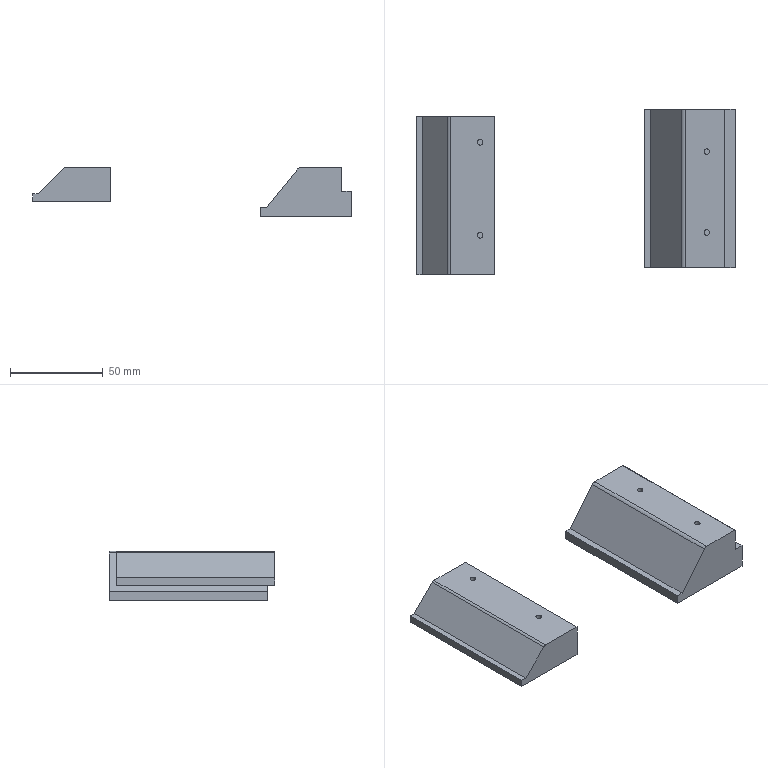NC program | NX | posted with a generic post | part box 171.319 x 88.841 x 26.598 mm
Lines 1 to 984 of 3096:
N10 G17 G21 G94 G90
(FLOOR_WALL_COPY_COPY_1 , TOOL : D80)
N12 T19 M6
N14 G54
N16 G17 G0 G90 X91.5 Y0. S6500 M3
N18 G43 Z30. H19
N20 Z3.
N22 G94 G1 Z0. F1500.
N24 X86.5
N26 X-86.5
N28 X-91.5
N30 Z3.
N32 G0 Z30.
N34 M5
(ADAPTIVE_MILLING_COPY , TOOL : D10)
N36 T15 M6
N38 G54
N40 G17 G0 G90 X3.849 Y-36.197 S9500 M3
N42 G43 Z30. H15
N44 Z-23.598
N46 G94 G1 Z-26.598 F1000.
N48 X4.379 Y-34.84 F3000.
N50 G3 X3.849 Y-33.55 R1.015
N52 X0.69 Y-32.906 R9.424
N54 X-10.806 Y-32.71 R185.073
N56 G1 X-16.206 Y-32.708
N58 X-43.706
N60 X-43.906 Y-32.706
N62 X-44.006 Y-32.702
N64 X-44.106 Y-32.696
N66 X-44.206 Y-32.687
N68 G2 X-48.539 Y-29.776 R6.033
N70 X-50.327 Y-24.206 R13.143
N72 X-50.675 Y-15.618 R79.626
N74 G1 X-50.681 Y-14.118
N76 X-50.686 Y-12.018
N78 X-50.689 Y-8.418
N80 X-50.69 Y5.282
N82 Y25.782
N84 X-50.689 Y25.882
N86 G2 X-48.028 Y30.358 R5.825
N88 X-42.511 Y32.287 R12.476
N90 X-33.926 Y32.674 R71.857
N92 G1 X-32.526 Y32.681
N94 X-30.726 Y32.686
N96 X-27.726 Y32.689
N98 X-20.226 Y32.691
N100 X43.774
N102 X43.874 Y32.69
N104 G2 X48.354 Y30.034 R5.824
N106 X50.271 Y24.618 R12.357
N108 X50.672 Y16.133 R68.209
N110 G1 X50.68 Y14.733
N112 X50.685 Y12.833
N114 X50.689 Y9.933
N116 X50.69 Y2.833
N118 Y-25.767
N120 Y-25.867
N122 G2 X48.204 Y-30.232 R5.74
N124 X42.726 Y-32.256 R11.985
N126 X33.943 Y-32.674 R68.16
N128 G1 X32.543 Y-32.681
N130 X30.543 Y-32.686
N132 X27.343 Y-32.689
N134 X18.843 Y-32.691
N136 X7.243
N138 X7.043 Y-32.689
N140 G2 X1.664 Y-32.223 R111.627
N142 G3 X-9.629 Y-31.926 R157.692
N144 G1 X-11.929 Y-31.921
N146 X-15.629 Y-31.918
N148 X-26.529 Y-31.917
N150 X-41.029
N152 X-41.229 Y-31.913
N154 X-41.429 Y-31.905
N156 G2 X-47.519 Y-28.063 R7.652
N158 X-49.458 Y-21.91 R15.376
N160 X-49.864 Y-12.224 R86.303
N162 G1 X-49.872 Y-10.624
N164 X-49.877 Y-8.424
N166 X-49.88 Y-4.924
N168 X-49.882 Y4.976
N170 Y22.976
N172 X-49.88 Y23.176
N174 G2 X-46.165 Y29.44 R7.571
N176 X-39.837 Y31.468 R15.23
N178 X-29.75 Y31.867 R92.737
N180 G1 X-28.05 Y31.874
N182 X-25.65 Y31.879
N184 X-21.45 Y31.881
N186 X-0.55 Y31.882
N188 X41.05
N190 X41.15 Y31.881
N192 G2 X47.426 Y28.187 R7.56
N194 X49.45 Y21.962 R15.013
N196 X49.864 Y12.277 R83.801
N198 G1 X49.872 Y10.677
N200 X49.877 Y8.477
N202 X49.88 Y4.977
N204 X49.882 Y-4.623
N206 Y-23.023
N208 X49.881 Y-23.123
N210 G2 X46.126 Y-29.468 R7.59
N212 X39.791 Y-31.474 R15.278
N214 X30.104 Y-31.865 R90.251
N216 G1 X28.604 Y-31.873
N218 X26.404 Y-31.878
N220 X22.804 Y-31.881
N222 X12.204 Y-31.882
N224 X9.304
N226 X8.904 Y-31.879
N228 G2 X0.82 Y-31.382 R206.463
N230 G3 X-15.076 Y-31.129 R317.576
N232 G1 X-20.176 Y-31.126
N234 X-38.376 Y-31.125
N236 X-38.676 Y-31.123
N238 X-38.876 Y-31.12
N240 X-39.076 Y-31.116
N242 X-39.176 Y-31.113
N244 G2 X-44.362 Y-29.256 R8.631
N246 X-46.183 Y-28.087 R5.15
N248 X-47.547 Y-25.613 R6.288
N250 X-48.893 Y-17.349 R30.717
N252 X-49.072 Y-1.551 R382.832
N254 G1 X-49.073 Y9.649
N256 Y20.749
N258 X-49.07 Y20.949
N260 X-49.065 Y21.149
N262 X-49.057 Y21.348
N264 X-49.053 Y21.448
N266 G2 X-47.297 Y26.261 R8.566
N268 X-46.087 Y28.183 R5.256
N270 X-43.613 Y29.547 R6.288
N272 X-35.449 Y30.89 R30.764
N274 X-19.451 Y31.072 R379.572
N276 G1 X-7.651 Y31.074
N278 X38.749 Y31.073
N280 X38.949 Y31.071
N282 X39.148 Y31.065
N284 X39.348 Y31.058
N286 X39.448 Y31.053
N288 G2 X44.259 Y29.298 R8.534
N290 X46.183 Y28.087 R5.258
N292 X47.547 Y25.613 R6.288
N294 X48.898 Y17.249 R30.761
N296 X49.071 Y3.451 R338.758
N298 G1 X49.073 Y-2.849
N300 Y-20.649
N302 X49.07 Y-20.949
N304 X49.066 Y-21.148
N306 X49.057 Y-21.348
N308 X49.053 Y-21.448
N310 G2 X47.296 Y-26.264 R8.56
N312 X46.087 Y-28.183 R5.252
N314 X43.613 Y-29.547 R6.288
N316 X35.548 Y-30.88 R30.187
N318 X20.651 Y-31.072 R329.152
N320 X8.052 Y-31.006 R402.069
N322 G3 X-13.533 Y-30.342 R296.331
N324 G1 X-16.533 Y-30.337
N326 X-21.633 Y-30.335
N328 X-35.733 Y-30.333
N330 X-36.433 Y-30.329
N332 X-36.733 Y-30.327
N334 X-37.032 Y-30.321
N336 G2 X-40.961 Y-29.65 R14.479
N338 X-43.896 Y-29.448 R12.283
N340 G1 X-44.451 Y-29.219
N342 X-44.796 Y-29.08
N344 X-45.13 Y-28.918
N346 G2 X-47.448 Y-25.896 R5.486
N348 X-47.697 Y-22.867 R18.604
N350 X-48.25 Y-7.182 R183.364
N352 G1 X-48.257 Y-4.982
N354 X-48.262 Y-1.882
N356 X-48.264 Y3.718
N358 Y18.618
N360 X-48.263 Y18.818
N362 X-48.26 Y19.018
N364 G2 X-47.65 Y22.838 R14.478
N366 X-47.448 Y25.896 R12.942
N368 G1 X-47.295 Y26.266
N370 G3 X-49.411 Y26.697 R-1.1
N372 G1 X-49.85 Y-23.856
N374 G3 X-48.758 Y-24.964 R1.1
N376 X-47.65 Y-23.866 R1.1
N378 G1 Y22.934
N380 G2 X-47.448 Y25.896 R12.58
N382 X-45.011 Y28.986 R5.459
N384 G1 X-43.896 Y29.448
N386 G2 X-40.967 Y29.69 R17.021
N388 X-24.282 Y30.254 R190.159
N390 G1 X-21.782 Y30.26
N392 X-17.882 Y30.263
N394 X-7.982 Y30.265
N396 X36.618
N398 X36.818 Y30.263
N400 X37.018 Y30.26
N402 G2 X40.843 Y29.65 R14.669
N404 X43.896 Y29.448 R12.914
N406 G1 X44.266 Y29.295
N408 G3 X44.693 Y31.411 R-1.1
N410 G1 X-41.86 Y31.85
N412 G3 X-42.964 Y30.754 R1.1
N414 X-41.866 Y29.65 R1.1
N416 G1 X40.934
N418 G2 X43.896 Y29.448 R12.58
N420 X46.986 Y27.011 R5.459
N422 G1 X47.448 Y25.896
N424 G2 X47.697 Y22.867 R18.604
N426 X48.254 Y6.082 R193.831
N428 G1 X48.26 Y3.482
N430 X48.263 Y-0.418
N432 X48.264 Y-11.018
N434 Y-18.618
N436 X48.263 Y-18.818
N438 X48.26 Y-19.018
N440 G2 X47.65 Y-22.84 R14.597
N442 X47.448 Y-25.896 R12.933
N444 G1 X47.295 Y-26.266
N446 G3 X49.411 Y-26.697 R-1.1
N448 G1 X49.85 Y23.856
N450 G3 X48.758 Y24.964 R1.1
N452 X47.65 Y23.866 R1.1
N454 G1 Y-22.934
N456 G2 X47.448 Y-25.896 R12.58
N458 X45.011 Y-28.986 R5.459
N460 G1 X43.896 Y-29.448
N462 G2 X40.967 Y-29.69 R17.021
N464 X24.381 Y-30.254 R192.172
N466 X8.383 Y-30.18 R503.879
N468 G3 X-4.026 Y-29.65 R498.123
N470 G1 X-41.026
N472 G3 X-42.124 Y-30.752 R1.1
N474 X-41.026 Y-31.85 R1.1
N476 G1 X41.866
N478 G3 X42.964 Y-30.748 R1.1
N480 X41.866 Y-29.65 R1.1
N482 G1 X-4.034
N484 G3 X-5.032 Y-30.5 R1.016
N486 G1 X-5.282 Y-32.063
N488 Z-23.598
N490 G0 Z30.
N492 X50.15 Y-19.797
N494 Z-17.688
N496 G1 Z-20.688 F1000.
N498 X48.446 Y-20.027 F3000.
N500 G3 X47.579 Y-20.9 R1.017
N502 G2 X46.954 Y-23.849 R14.313
N504 X42.853 Y-27.594 R7.265
N506 X36.792 Y-28.764 R19.282
N508 X23.295 Y-28.94 R270.559
N510 G1 X11.595 Y-28.941
N512 X-39.805
N514 X-40.005 Y-28.939
N516 X-40.105 Y-28.936
N518 X-40.305 Y-28.926
N520 X-40.404 Y-28.919
N522 G2 X-44.833 Y-25.85 R5.86
N524 G1 X-44.932 Y-25.676
N526 X-45.027 Y-25.5
N528 X-45.118 Y-25.322
N530 X-45.163 Y-25.233
N532 X-45.249 Y-25.052
N534 X-45.29 Y-24.961
N536 X-45.371 Y-24.778
N538 X-45.416 Y-24.689
N540 X-45.468 Y-24.604
N542 X-45.528 Y-24.523
N544 G2 X-47.488 Y-21.617 R5.52
N546 G1 X-47.576 Y-20.922
N548 G3 X-49.48 Y-20.639 R1.001
N550 G1 X-49.568 Y-20.962 Z-20.671
N552 X-49.61 Y-21.294 Z-20.654
N554 X-49.784 Y-22.612 Z-20.588
N556 X-49.897 Y-23.443
N558 X-49.994 Y-24.277
N560 G3 X-49.826 Y-24.819 R1.053
N562 G1 X-48.816 Y-26.342
N564 X-47.788 Y-27.852
N566 G3 X-45.522 Y-30.062 R10.243
N568 X-43.944 Y-31.048 R10.274
N570 X-40.335 Y-31.844 R8.917
N572 X-24.721 Y-32.034 R967.791
N574 G1 X31.754 Y-32.273
N576 G3 X42.415 Y-31.058 R45.907
N578 G1 X44.084 Y-30.671
N580 X45.748 Y-30.259
N582 G3 X48.693 Y-27.715 R4.933
N584 G1 X49.239 Y-26.601
N586 X49.765 Y-25.478
N588 X49.804 Y-25.269
N590 X49.805 Y-25.056
N592 X49.581 Y-23.175
N594 X49.497 Y-22.429 Z-20.625
N596 X49.389 Y-21.687 Z-20.663
N598 X49.287 Y-21.461 Z-20.675
N600 X49.137 Y-21.262 Z-20.688
N602 G3 X47.462 Y-21.713 R1.002
N604 G2 X45.021 Y-24.946 R5.92
N606 X38.182 Y-27.576 R15.275
N608 X28.705 Y-28.104 R68.799
N610 G1 X27.505 Y-28.114
N612 X26.005 Y-28.121
N614 X23.905 Y-28.127
N616 X20.705 Y-28.13
N618 X13.405 Y-28.132
N620 X-37.295
N622 G2 X-42.145 Y-26.272 R7.713
N624 G3 X-43.27 Y-25.451 R5.42
N626 G2 X-45.691 Y-24.364 R4.847
N628 G3 X-47.175 Y-25.643 R1.
N630 G1 X-46.828 Y-26.095 Z-20.659
N632 X-46.458 Y-26.529 Z-20.631
N634 X-45.907 Y-27.188 Z-20.588
N636 X-44.751 Y-28.556
N638 X-44.526 Y-28.711
N640 X-43.031 Y-29.46
N642 X-41.529 Y-30.195
N644 G3 X-36.731 Y-31.211 R11.921
N646 G1 X29.266
N648 G3 X38.198 Y-30.646 R72.394
N650 X43.223 Y-29.491 R28.954
N652 G1 X46.096 Y-28.55
N654 G3 X46.733 Y-27.918 R1.015
N656 G1 X47.269 Y-26.314
N658 X47.491 Y-25.664 Z-20.622
N660 X47.694 Y-25.007 Z-20.656
N662 G3 X47.604 Y-24.398 Z-20.688 R1.045
N664 X46.096 Y-24.05 R1.003
N666 G2 X43.479 Y-25.441 R5.812
N668 X31.346 Y-27.21 R45.189
N670 X14.047 Y-27.323 R764.399
N672 G1 X-34.853 Y-27.324
N674 X-35.153 Y-27.321
N676 X-35.253 Y-27.319
N678 X-35.453 Y-27.312
N680 X-35.553 Y-27.308
N682 G2 X-40.595 Y-25.814 R12.608
N684 G3 X-41.347 Y-25.538 R3.965
N686 G2 X-43.427 Y-25.412 R9.987
N688 G3 X-43.574 Y-27.602 R-1.1
N690 G1 X43.918 Y-27.555
N692 G3 X43.769 Y-25.365 R-1.1
N694 G2 X41.066 Y-25.584 R19.392
N696 X24.702 Y-26.49 R133.122
N698 G1 X23.102 Y-26.499
N700 X21.102 Y-26.506
N702 X18.302 Y-26.511
N704 X13.702 Y-26.514
N706 X-2.398 Y-26.515
N708 X-32.798
N710 G2 X-38.59 Y-25.544 R18.348
N712 G1 X-38.646 Y-25.538
N714 X-41.446
N716 G3 X-42.544 Y-26.64 R1.1
N718 X-41.446 Y-27.738 R1.1
N720 G1 X41.965
N722 G3 X43.063 Y-26.636 R1.1
N724 X41.965 Y-25.538 R1.1
N726 X25.466 Y-25.674 R601.078
N728 G1 X23.566 Y-25.685
N730 X21.266 Y-25.694
N732 X18.566 Y-25.7
N734 X14.666 Y-25.704
N736 X7.066 Y-25.706
N738 X-30.834 Y-25.707
N740 G2 X-33.987 Y-25.538 R35.236
N742 G1 X-38.687
N744 G3 X-39.785 Y-26.64 R1.1
N746 X-38.687 Y-27.738 R1.1
N748 G1 X33.165
N750 G3 X34.263 Y-26.636 R1.1
N752 X33.165 Y-25.538 R1.1
N754 G1 X-34.035
N756 G3 X-35.034 Y-26.399 R1.016
N758 G1 X-35.277 Y-28.021
N760 Z-17.688
N762 G0 Z30.
N764 X50.15 Y-18.954
N766 Z-16.702
N768 G1 Z-19.702 F1000.
N770 X48.445 Y-19.193 F3000.
N772 G3 X47.584 Y-20.066 R1.017
N774 G2 X46.926 Y-22.191 R5.216
N776 X43.769 Y-24.568 R5.484
N778 G1 X42.535 Y-24.735
N780 X42.465 Y-24.74
N782 X-42.465
N784 X-42.535 Y-24.735
N786 G2 X-46.096 Y-23.253 R5.566
N788 X-47.488 Y-20.819 R5.729
N790 G1 X-47.576 Y-20.125
N792 G3 X-48.443 Y-19.252 R1.017
N794 G1 X-50.146 Y-19.022
N796 Z-16.702
N798 G0 Z30.
N800 X50.15 Y-18.156
N802 Z-15.717
N804 G1 Z-18.717 F1000.
N806 X48.445 Y-18.396 F3000.
N808 G3 X47.584 Y-19.268 R1.017
N810 G2 X46.926 Y-21.394 R5.216
N812 X43.769 Y-23.77 R5.484
N814 G1 X42.535 Y-23.938
N816 X42.465 Y-23.942
N818 X-42.465
N820 X-42.535 Y-23.938
N822 G2 X-46.096 Y-22.455 R5.566
N824 X-47.488 Y-20.021 R5.729
N826 G1 X-47.576 Y-19.327
N828 G3 X-48.443 Y-18.454 R1.017
N830 G1 X-50.146 Y-18.224
N832 Z-15.717
N834 G0 Z30.
N836 X50.15 Y-17.358
N838 Z-14.732
N840 G1 Z-17.732 F1000.
N842 X48.445 Y-17.598 F3000.
N844 G3 X47.584 Y-18.47 R1.017
N846 G2 X46.926 Y-20.596 R5.216
N848 X43.769 Y-22.972 R5.484
N850 G1 X42.535 Y-23.14
N852 X42.465 Y-23.145
N854 X-42.465
N856 X-42.535 Y-23.14
N858 G2 X-46.096 Y-21.657 R5.566
N860 X-47.488 Y-19.224 R5.729
N862 G1 X-47.589 Y-18.43
N864 G3 X-48.444 Y-17.559 R1.017
N866 G1 X-50.146 Y-17.309
N868 Z-14.732
N870 G0 Z30.
N872 X50.15 Y-16.561
N874 Z-13.747
N876 G1 Z-16.747 F1000.
N878 X48.445 Y-16.8 F3000.
N880 G3 X47.584 Y-17.673 R1.017
N882 G2 X46.926 Y-19.798 R5.216
N884 X43.769 Y-22.174 R5.484
N886 G1 X42.535 Y-22.342
N888 X42.465 Y-22.347
N890 X-42.465
N892 X-42.535 Y-22.342
N894 G2 X-46.096 Y-20.86 R5.566
N896 X-47.488 Y-18.426 R5.729
N898 G1 X-47.576 Y-17.731
N900 G3 X-48.443 Y-16.858 R1.017
N902 G1 X-50.146 Y-16.628
N904 Z-13.747
N906 G0 Z30.
N908 X50.15 Y-15.763
N910 Z-12.762
N912 G1 Z-15.762 F1000.
N914 X48.445 Y-16.002 F3000.
N916 G3 X47.584 Y-16.875 R1.017
N918 G2 X46.926 Y-19. R5.216
N920 X43.769 Y-21.377 R5.484
N922 G1 X42.535 Y-21.544
N924 X42.465 Y-21.549
N926 X-42.465
N928 X-42.535 Y-21.544
N930 G2 X-46.096 Y-20.062 R5.566
N932 X-47.488 Y-17.628 R5.729
N934 G1 X-47.576 Y-16.934
N936 G3 X-48.443 Y-16.061 R1.017
N938 G1 X-50.146 Y-15.831
N940 Z-12.762
N942 G0 Z30.
N944 X50.15 Y-14.965
N946 Z-11.777
N948 G1 Z-14.777 F1000.
N950 X48.445 Y-15.205 F3000.
N952 G3 X47.584 Y-16.077 R1.017
N954 G2 X46.926 Y-18.203 R5.216
N956 X43.769 Y-20.579 R5.484
N958 G1 X42.535 Y-20.747
N960 X42.465 Y-20.751
N962 X-42.465
N964 X-42.535 Y-20.747
N966 G2 X-46.096 Y-19.264 R5.566
N968 X-47.488 Y-16.83 R5.729
N970 G1 X-47.576 Y-16.136
N972 G3 X-48.443 Y-15.263 R1.017
N974 G1 X-50.146 Y-15.033
N976 Z-11.777
N978 G0 Z30.
N980 X50.15 Y-14.167
N982 Z-10.792
N984 G1 Z-13.792 F1000.
N986 X48.445 Y-14.407 F3000.
N988 G3 X47.584 Y-15.279 R1.017
N990 G2 X46.926 Y-17.405 R5.216
N992 X43.769 Y-19.781 R5.484
N994 G1 X42.535 Y-19.949
N996 X42.465 Y-19.954
N998 X-42.465
N1000 X-42.535 Y-19.949
N1002 G2 X-46.096 Y-18.466 R5.566
N1004 X-47.488 Y-16.033 R5.729
N1006 G1 X-47.576 Y-15.338
N1008 G3 X-48.443 Y-14.465 R1.017
N1010 G1 X-50.146 Y-14.235
N1012 Z-10.792
N1014 G0 Z30.
N1016 X-50.15 Y18.639
N1018 Z-9.849
N1020 G1 Z-12.849 F1000.
N1022 X-48.443 Y18.901 F3000.
N1024 G3 X-47.595 Y19.767 R1.017
N1026 G2 X-47.18 Y21.911 R20.723
N1028 X-44.025 Y26.738 R6.187
N1030 X-38.319 Y28.431 R13.772
N1032 X-28.928 Y28.742 R99.181
N1034 G1 X-26.928 Y28.749
N1036 X-23.628 Y28.754
N1038 X-13.928 Y28.76
N1040 X39.872 Y28.789
N1042 X39.972 Y28.788
N1044 X40.172 Y28.778
N1046 G2 X44.508 Y26.033 R6.034
N1048 X45.813 Y23.343 R11.987
N1050 X46.986 Y21.858 R22.085
N1052 X47.588 Y19.818 R5.323
N1054 G3 X49.497 Y19.55 R1.001
N1056 G1 X49.58 Y19.867 Z-12.833
N1058 X49.623 Y20.191 Z-12.816
N1060 X49.809 Y21.523 Z-12.749
N1062 X49.926 Y22.334
N1064 X50.024 Y23.147
N1066 G3 X49.838 Y23.715 R1.047
N1068 G1 X46.205 Y28.795
N1070 X45.92 Y29.164
N1072 X45.622 Y29.523
N1074 X45.276 Y29.831
N1076 X44.895 Y30.091
N1078 X43.815 Y30.709
N1080 X42.707 Y31.275
N1082 G3 X41.515 Y31.577 R3.614
N1084 X34.661 Y31.939 R133.44
N1086 G1 X9.042 Y32.517
N1088 G3 X-24.687 Y32.138 R502.521
N1090 G1 X-38.212 Y31.528
N1092 G3 X-44.603 Y30.047 R18.169
N1094 G1 X-45.933 Y29.454
N1096 G3 X-48.68 Y26.678 R6.302
N1098 G1 X-49.698 Y24.64
N1100 G3 X-49.794 Y24.054 R1.048
N1102 G1 X-49.541 Y22.254
N1104 X-49.332 Y20.846 Z-12.82
N1106 G3 X-49.025 Y20.368 Z-12.849 R1.053
N1108 X-47.448 Y20.743 R1.003
N1110 G2 X-44.411 Y24.802 R8.596
N1112 X-38.169 Y27.327 R14.066
N1114 X-29.197 Y27.907 R59.266
N1116 G1 X-28.097 Y27.919
N1118 X-26.897 Y27.928
N1120 X-25.297 Y27.936
N1122 X-23.097 Y27.942
N1124 X-19.497 Y27.947
N1126 X-8.897 Y27.954
N1128 X37.103 Y27.979
N1130 X37.203
N1132 X37.403 Y27.973
N1134 X37.603 Y27.963
N1136 G2 X42.613 Y25.532 R7.701
N1138 G3 X43.817 Y24.337 R17.394
N1140 G1 X43.897 Y24.295
N1142 X45.011 Y23.833
N1144 X45.13 Y23.765
N1146 X46.082 Y23.034
N1148 G3 X47.615 Y23.445 R1.003
N1150 X47.547 Y24.377 Z-12.801 R1.136
N1152 G1 X47.158 Y25.337 Z-12.749
N1154 X46.783 Y26.278
N1156 X46.388 Y27.211
N1158 X46.25 Y27.387
N1160 X46.082 Y27.534
N1162 X45.043 Y28.226
N1164 X43.977 Y28.877
N1166 G3 X40.804 Y30.332 R28.728
N1168 X36.896 Y31.028 R12.549
N1170 G1 X-7.466 Y31.813
N1172 G3 X-28.684 Y31.194 R228.157
N1174 G1 X-37.408 Y30.53
N1176 G3 X-44.492 Y28.354 R17.09
N1178 G1 X-48.083 Y26.323
N1180 G3 X-48.59 Y25.494 R1.014
N1182 G1 X-48.66 Y23.826
N1184 X-48.693 Y23.147 Z-12.783
N1186 X-48.705 Y22.467 Z-12.817
N1188 G3 X-48.438 Y21.897 Z-12.849 R1.043
N1190 X-46.918 Y21.976 R1.004
N1192 G2 X-44.206 Y24.234 R5.794
N1194 X-34.31 Y26.825 R25.686
N1196 X-22.717 Y27.129 R159.214
N1198 G1 X-20.217 Y27.135
N1200 X-16.017 Y27.141
N1202 X-1.917 Y27.15
N1204 X31.583 Y27.168
N1206 X33.183 Y27.174
N1208 X34.283
N1210 G2 X40.88 Y25.236 R10.694
N1212 G3 X42.186 Y24.514 R5.424
N1214 G2 X43.989 Y24.256 R9.366
N1216 G3 X45.349 Y24.967 R1.003
N1218 X45.123 Y25.847 Z-12.802 R1.046
N1220 G1 X44.499 Y26.703 Z-12.749
N1222 X43.389 Y28.222
N1224 G3 X42.824 Y28.603 R1.038
N1226 G1 X39.036 Y29.538
N1228 G3 X33.636 Y30.13 R26.099
N1230 G1 X-10.112 Y30.29
N1232 G3 X-32.982 Y29.968 R706.907
N1234 X-38.296 Y29.34 R42.759
N1236 X-43.847 Y28.179 R110.579
N1238 X-44.438 Y27.789 R1.031
N1240 G1 X-45.474 Y26.355
N1242 X-45.886 Y25.79 Z-12.784
N1244 X-46.283 Y25.214 Z-12.819
N1246 G3 X-46.386 Y24.632 Z-12.849 R1.048
N1248 X-45.011 Y23.833 R1.003
N1250 G2 X-42.776 Y24.478 R6.015
N1252 X-28.617 Y26.235 R61.253
N1254 X-11.018 Y26.335 R827.99
N1256 G1 X28.982 Y26.358
N1258 X30.082 Y26.364
N1260 X31.682 Y26.365
N1262 X32.382 Y26.368
N1264 X32.982 Y26.364
N1266 X33.182 Y26.36
N1268 G2 X39.347 Y24.839 R14.909
N1270 G3 X40.307 Y24.496 R6.185
N1272 G1 X42.307
N1274 G3 X43.405 Y25.598 R1.1
N1276 X42.306 Y26.696 R1.1
N1278 G1 X-43.315 Y26.599
N1280 G3 X-43.17 Y24.408 R-1.1
N1282 G2 X-40.666 Y24.506 R16.266
N1284 X-32.898 Y25.204 R931.865
N1286 X-17.604 Y25.517 R261.002
N1288 G1 X-14.104 Y25.523
N1290 X-7.304 Y25.529
N1292 X26.296 Y25.548
N1294 X27.396 Y25.554
N1296 X28.996 Y25.556
N1298 X30.096 Y25.561
N1300 G2 X37.482 Y24.506 R20.965
N1302 G1 X37.571 Y24.496
N1304 X40.371
N1306 G3 X41.469 Y25.598 R1.1
N1308 X40.371 Y26.696 R1.1
N1310 G1 X-40.966
N1312 G3 X-42.064 Y25.594 R1.1
N1314 X-40.966 Y24.496 R1.1
N1316 X-24.267 Y24.668 R538.832
N1318 G1 X-22.568 Y24.682
N1320 X-20.768 Y24.693
N1322 X-18.668 Y24.703
N1324 X-15.868 Y24.71
N1326 X-11.768 Y24.716
N1328 X-3.168 Y24.723
N1330 X23.632 Y24.738
N1332 X24.832 Y24.745
N1334 X26.332 Y24.746
N1336 X27.332 Y24.752
N1338 X28.432
N1340 X29.232 Y24.751
N1342 G2 X33.158 Y24.496 R32.119
N1344 G1 X37.658
N1346 G3 X38.756 Y25.598 R1.1
N1348 X37.658 Y26.696 R1.1
N1350 G1 X-32.666
N1352 G3 X-33.764 Y25.594 R1.1
N1354 X-32.666 Y24.496 R1.1
N1356 G1 X33.234
N1358 G3 X34.233 Y25.356 R1.016
N1360 G1 X34.48 Y26.996
N1362 Z-9.849
N1364 G0 Z30.
N1366 X50.15 Y-12.581
N1368 Z-8.821
N1370 G1 Z-11.821 F1000.
N1372 X48.445 Y-12.819 F3000.
N1374 G3 X47.583 Y-13.691 R1.017
N1376 G2 X46.926 Y-15.809 R5.209
N1378 X43.711 Y-18.214 R5.547
N1380 X37.496 Y-19.123 R24.164
N1382 X18.798 Y-19.243 R624.136
N1384 G1 X-39.902 Y-19.238
N1386 X-40.002 Y-19.237
N1388 X-40.102 Y-19.232
N1390 X-40.202 Y-19.226
N1392 X-40.302 Y-19.217
N1394 G2 X-42.633 Y-18.375 R5.673
N1396 G3 X-43.901 Y-18.15 R36.081
N1398 G2 X-46.994 Y-15.691 R5.484
N1400 X-47.576 Y-13.743 R5.242
N1402 G3 X-49.412 Y-13.332 R1.001
N1404 X-49.603 Y-13.972 Z-11.788 R1.681
N1406 G1 X-49.838 Y-15.278 Z-11.721
N1408 X-49.991 Y-16.095
N1410 X-50.119 Y-16.915
N1412 G3 X-49.826 Y-17.64 R1.026
N1414 G1 X-49.002 Y-18.466
N1416 X-48.166 Y-19.281
N1418 G3 X-45.389 Y-20.862 R7.819
N1420 G1 X-44.055 Y-21.286
N1422 X-42.705 Y-21.658
N1424 G3 X-38.096 Y-22.206 R20.616
N1426 G1 X8.103 Y-22.384
N1428 X13.44 Y-22.396
N1430 X18.776 Y-22.378
N1432 X24.113 Y-22.343
N1434 X29.449 Y-22.277
N1436 X38.769 Y-22.149
N1438 G3 X41.445 Y-21.854 R14.548
N1440 G1 X42.9 Y-21.542
N1442 X43.14 Y-21.418
N1444 X44.249 Y-20.639
N1446 X45.885 Y-19.489 Z-11.821
N1448 G3 X45.525 Y-17.611 R1.008
N1450 G1 X45.268 Y-17.617
N1452 X45.019 Y-17.681
N1454 X43.901 Y-18.15
N1456 X43.769 Y-18.186
N1458 X42.535 Y-18.353
N1460 X42.465 Y-18.358
N1462 G3 X28.865 Y-18.426 R865.463
N1464 G1 X26.465 Y-18.43
N1466 X22.465 Y-18.433
N1468 X10.765 Y-18.434
N1470 X-37.035 Y-18.43
N1472 X-37.235 Y-18.429
N1474 X-37.435 Y-18.423
N1476 X-37.635 Y-18.413
N1478 X-37.734 Y-18.407
N1480 X-37.934 Y-18.391
N1482 X-38.232 Y-18.361
N1484 X-38.253 Y-18.358
N1486 X-42.465
N1488 X-42.535 Y-18.353
N1490 X-42.832 Y-18.313
N1492 G3 X-42.981 Y-20.503 R-1.1
N1494 G1 X36.164 Y-20.558
N1496 G3 X37.263 Y-19.457 R1.1
N1498 X36.165 Y-18.358 R1.1
N1500 G1 X-38.335
N1502 G3 X-39.334 Y-19.519 R1.014
N1504 G1 X-39.133 Y-20.85
N1506 Z-8.821
N1508 G0 Z30.
N1510 X50.15 Y-11.774
N1512 Z-7.836
N1514 G1 Z-10.836 F1000.
N1516 X48.445 Y-12.014 F3000.
N1518 G3 X47.584 Y-12.886 R1.017
N1520 G2 X46.926 Y-15.012 R5.216
N1522 X43.769 Y-17.388 R5.484
N1524 G1 X42.535 Y-17.556
N1526 X42.465 Y-17.561
N1528 X-42.465
N1530 X-42.535 Y-17.556
N1532 G2 X-46.096 Y-16.073 R5.566
N1534 X-47.488 Y-13.639 R5.729
N1536 G1 X-47.589 Y-12.846
N1538 G3 X-48.444 Y-11.974 R1.017
N1540 G1 X-50.146 Y-11.724
N1542 Z-7.836
N1544 G0 Z30.
N1546 X50.15 Y-10.976
N1548 Z-6.851
N1550 G1 Z-9.851 F1000.
N1552 X48.445 Y-11.216 F3000.
N1554 G3 X47.584 Y-12.088 R1.017
N1556 G2 X46.926 Y-14.214 R5.216
N1558 X43.769 Y-16.59 R5.484
N1560 G1 X42.535 Y-16.758
N1562 X42.465 Y-16.763
N1564 X-42.465
N1566 X-42.535 Y-16.758
N1568 G2 X-46.096 Y-15.275 R5.566
N1570 X-47.488 Y-12.842 R5.729
N1572 G1 X-47.576 Y-12.147
N1574 G3 X-48.443 Y-11.274 R1.017
N1576 G1 X-50.146 Y-11.044
N1578 Z-6.851
N1580 G0 Z30.
N1582 X50.15 Y-10.13
N1584 Z-5.866
N1586 G1 Z-8.866 F1000.
N1588 X48.446 Y-10.369 F3000.
N1590 G3 X47.584 Y-11.248 R1.017
N1592 G2 X46.938 Y-13.372 R5.224
N1594 X43.777 Y-15.783 R5.521
N1596 G1 X42.537 Y-15.96
N1598 X42.463 Y-15.965
N1600 X-42.463
N1602 X-42.537 Y-15.96
N1604 G2 X-46.109 Y-14.445 R5.601
N1606 X-47.494 Y-11.989 R5.768
N1608 G1 X-47.579 Y-11.294
N1610 G3 X-48.445 Y-10.415 R1.017
N1612 G1 X-50.146 Y-10.183
N1614 Z-5.866
N1616 G0 Z30.
N1618 X50.15 Y-9.386
N1620 Z-4.881
N1622 G1 Z-7.881 F1000.
N1624 X48.445 Y-9.624 F3000.
N1626 G3 X47.583 Y-10.497 R1.017
N1628 G2 X46.926 Y-12.618 R5.213
N1630 X43.769 Y-14.995 R5.484
N1632 G1 X42.535 Y-15.163
N1634 X42.465 Y-15.167
N1636 X-42.465
N1638 X-42.535 Y-15.163
N1640 G2 X-46.096 Y-13.68 R5.566
N1642 X-47.488 Y-11.246 R5.729
N1644 G1 X-47.576 Y-10.552
N1646 G3 X-48.443 Y-9.679 R1.017
N1648 G1 X-50.146 Y-9.449
N1650 Z-4.881
N1652 G0 Z30.
N1654 X50.15 Y-8.583
N1656 Z-3.896
N1658 G1 Z-6.896 F1000.
N1660 X48.445 Y-8.823 F3000.
N1662 G3 X47.584 Y-9.695 R1.017
N1664 G2 X46.926 Y-11.821 R5.216
N1666 X43.769 Y-14.197 R5.484
N1668 G1 X42.535 Y-14.365
N1670 X42.465 Y-14.37
N1672 X-42.465
N1674 X-42.535 Y-14.365
N1676 G2 X-46.096 Y-12.882 R5.566
N1678 X-47.488 Y-10.448 R5.729
N1680 G1 X-47.576 Y-9.754
N1682 G3 X-48.443 Y-8.881 R1.017
N1684 G1 X-50.146 Y-8.651
N1686 Z-3.896
N1688 G0 Z30.
N1690 X50.15 Y-7.785
N1692 Z-2.911
N1694 G1 Z-5.911 F1000.
N1696 X48.445 Y-8.025 F3000.
N1698 G3 X47.584 Y-8.897 R1.017
N1700 G2 X46.926 Y-11.023 R5.216
N1702 X43.769 Y-13.399 R5.484
N1704 G1 X42.535 Y-13.567
N1706 X42.465 Y-13.572
N1708 X-42.465
N1710 X-42.535 Y-13.567
N1712 G2 X-46.096 Y-12.084 R5.566
N1714 X-47.488 Y-9.651 R5.729
N1716 G1 X-47.576 Y-8.956
N1718 G3 X-48.443 Y-8.083 R1.017
N1720 G1 X-50.146 Y-7.853
N1722 Z-2.911
N1724 G0 Z30.
N1726 X50.15 Y-6.988
N1728 Z-1.926
N1730 G1 Z-4.926 F1000.
N1732 X48.445 Y-7.227 F3000.
N1734 G3 X47.584 Y-8.1 R1.017
N1736 G2 X46.926 Y-10.225 R5.216
N1738 X43.769 Y-12.602 R5.484
N1740 G1 X42.535 Y-12.769
N1742 X42.465 Y-12.774
N1744 X-42.465
N1746 X-42.535 Y-12.769
N1748 G2 X-46.096 Y-11.287 R5.566
N1750 X-47.488 Y-8.853 R5.729
N1752 G1 X-47.576 Y-8.159
N1754 G3 X-48.443 Y-7.285 R1.017
N1756 G1 X-50.146 Y-7.056
N1758 Z-1.926
N1760 G0 Z30.
N1762 X50.15 Y-6.19
N1764 Z-0.94
N1766 G1 Z-3.94 F1000.
N1768 X48.445 Y-6.429 F3000.
N1770 G3 X47.584 Y-7.302 R1.017
N1772 G2 X46.926 Y-9.427 R5.216
N1774 X43.769 Y-11.804 R5.484
N1776 G1 X42.535 Y-11.972
N1778 X42.465 Y-11.976
N1780 X-42.465
N1782 X-42.535 Y-11.972
N1784 G2 X-46.096 Y-10.489 R5.566
N1786 X-47.488 Y-8.055 R5.729
N1788 G1 X-47.576 Y-7.361
N1790 G3 X-48.443 Y-6.488 R1.017
N1792 G1 X-50.146 Y-6.258
N1794 Z-0.94
N1796 G0 Z30.
N1798 X50.15 Y-5.392
N1800 Z0.045
N1802 G1 Z-2.955 F1000.
N1804 X48.445 Y-5.632 F3000.
N1806 G3 X47.584 Y-6.504 R1.017
N1808 G2 X46.926 Y-8.63 R5.216
N1810 X43.769 Y-11.006 R5.484
N1812 G1 X42.535 Y-11.174
N1814 X42.465 Y-11.179
N1816 X-42.465
N1818 X-42.535 Y-11.174
N1820 G2 X-46.096 Y-9.691 R5.566
N1822 X-47.488 Y-7.257 R5.729
N1824 G1 X-47.589 Y-6.464
N1826 G3 X-48.444 Y-5.592 R1.017
N1828 G1 X-50.146 Y-5.343
N1830 Z0.045
N1832 G0 Z30.
N1834 X50.15 Y-4.594
N1836 Z1.03
N1838 G1 Z-1.97 F1000.
N1840 X48.445 Y-4.834 F3000.
N1842 G3 X47.584 Y-5.706 R1.017
N1844 G2 X46.926 Y-7.832 R5.216
N1846 X43.769 Y-10.208 R5.484
N1848 G1 X42.535 Y-10.376
N1850 X42.465 Y-10.381
N1852 X-42.465
N1854 X-42.535 Y-10.376
N1856 G2 X-46.096 Y-8.893 R5.566
N1858 X-47.488 Y-6.46 R5.729
N1860 G1 X-47.576 Y-5.765
N1862 G3 X-48.443 Y-4.892 R1.017
N1864 G1 X-50.146 Y-4.662
N1866 Z1.03
N1868 G0 Z30.
N1870 M5
(ZLEVEL_PROFILE_COPY_1_COPY_COPY_1_COPY , TOOL : D10JING)
N1872 T14 M6
N1874 G54
N1876 G17 G0 G90 X44.122 Y-31.309 S9500 M3
N1878 G43 Z30. H14
N1880 Z-25.598
N1882 G94 G1 Z-26.598 F1000.
N1884 X43.366 Y-30.
N1886 G3 X42.5 Y-29.5 R1.
N1888 G1 X-42.5 F1200.
N1890 G2 X-47.5 Y-24.5 R5.
N1892 G1 Y24.5
N1894 G2 X-42.5 Y29.5 R5.
N1896 G1 X42.5
N1898 G2 X47.5 Y24.5 R5.
N1900 G1 Y-24.5
N1902 G2 X42.5 Y-29.5 R5.
N1904 G3 X41.634 Y-30. R1.
N1906 G1 X40.768 Y-31.5
N1908 Z-25.598
N1910 G0 Z30.
(FLOOR_WALL_1_COPY , TOOL : D10JING)
N1912 X-50.5 Y24.5
N1914 Z-10.
N1916 G1 Z-13. F1250.
N1918 X-47.5
N1920 X47.5
N1922 Y24.346
N1924 X-47.5
N1926 X-50.5
N1928 Z-10.
N1930 G0 Z30.
N1932 X50.5 Y-26.082
N1934 Z-18.598
N1936 G1 Z-21.598
N1938 X47.5
N1940 X-47.5
N1942 X-50.5
N1944 Z-18.598
N1946 G0 Z30.
N1948 M5